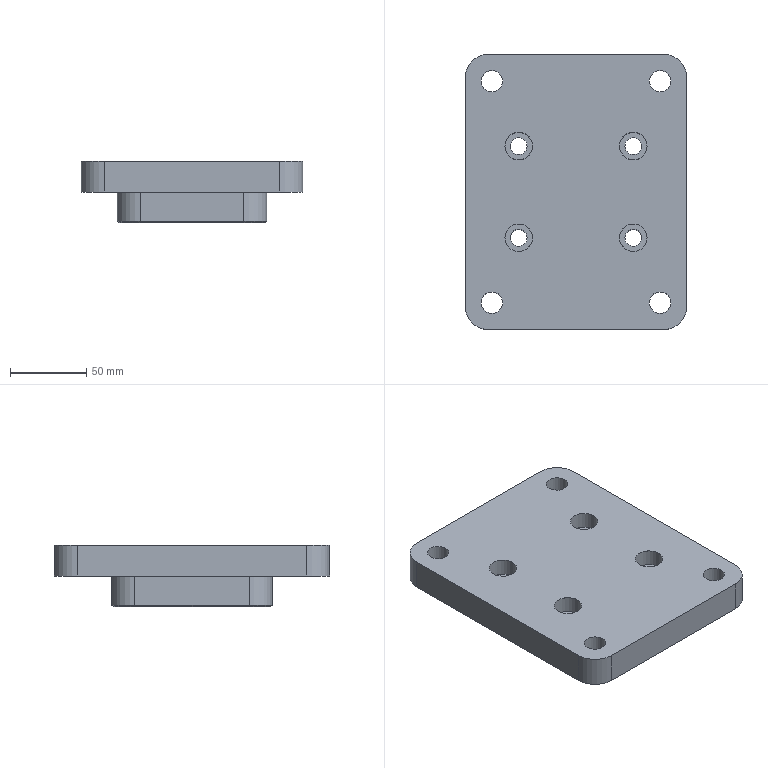NC program | NX | posted with a generic post | part box 145 x 180 x 40 mm
Lines 5548 to 5818 of 5818:
(HOLE_MILLING_COPY , TOOL : D10JING)
N11076 T11 M6
N11078 G54
N11080 G17 G0 G90 X-72.5 Y55. S5000 M3
N11082 G43 Z30. H11
N11084 Z0.5
N11086 G94 G3 X-73.5 Y54. R1. F1200.
N11088 X-72.5 Y53. R1.
N11090 X-72.5 Y53. Z-4.5 I0. J2.
N11092 X-72.5 Y53. Z-9.5 I0. J2.
N11094 X-72.5 Y53. Z-14.5 I0. J2.
N11096 X-72.5 Y53. Z-19.5 I0. J2.
N11098 X-71.324 Y53.382 Z-20. R2.
N11100 X-70.882 Y56.176 R2.
N11102 X-71.324 Y53.382 R-2.
N11104 X-71.103 Y54.779 R1.
N11106 X-72.5 Y55. R1.
N11108 G0 Z30.
N11110 X-30. Y37.5
N11112 Z0.5
N11114 G1 X-30.849 Y37.073
N11116 G3 X-30. Y33.5 R1.887
N11118 X-30. Y33.5 Z-4.5 I0. J4.
N11120 X-30. Y33.5 Z-9.5 I0. J4.
N11122 X-26.196 Y38.736 Z-11. R4.
N11124 X-31.236 Y41.304 R4.
N11126 X-26.196 Y38.736 R-4.
N11128 X-29.856 Y38.439 R1.887
N11130 G1 X-30. Y37.5
N11132 G0 Z30.
N11134 X30.
N11136 Z0.5
N11138 G1 X29.151 Y37.073
N11140 G3 X30. Y33.5 R1.887
N11142 X30. Y33.5 Z-4.5 I0. J4.
N11144 X30. Y33.5 Z-9.5 I0. J4.
N11146 X33.804 Y38.736 Z-11. R4.
N11148 X28.764 Y41.304 R4.
N11150 X33.804 Y38.736 R-4.
N11152 X30.144 Y38.439 R1.887
N11154 G1 X30. Y37.5
N11156 G0 Z30.
N11158 X72.5 Y55.
N11160 Z0.5
N11162 G3 X71.5 Y54. R1.
N11164 X72.5 Y53. R1.
N11166 X72.5 Y53. Z-4.5 I0. J2.
N11168 X72.5 Y53. Z-9.5 I0. J2.
N11170 X72.5 Y53. Z-14.5 I0. J2.
N11172 X72.5 Y53. Z-19.5 I0. J2.
N11174 X73.676 Y53.382 Z-20. R2.
N11176 X74.118 Y56.176 R2.
N11178 X73.676 Y53.382 R-2.
N11180 X73.897 Y54.779 R1.
N11182 X72.5 Y55. R1.
N11184 G0 Z30.
N11186 Y-55.
N11188 Z0.5
N11190 G3 X71.5 Y-56. R1.
N11192 X72.5 Y-57. R1.
N11194 X72.5 Y-57. Z-4.5 I0. J2.
N11196 X72.5 Y-57. Z-9.5 I0. J2.
N11198 X72.5 Y-57. Z-14.5 I0. J2.
N11200 X72.5 Y-57. Z-19.5 I0. J2.
N11202 X73.676 Y-56.618 Z-20. R2.
N11204 X74.118 Y-53.824 R2.
N11206 X73.676 Y-56.618 R-2.
N11208 X73.897 Y-55.221 R1.
N11210 X72.5 Y-55. R1.
N11212 G0 Z30.
N11214 X30. Y-37.5
N11216 Z0.5
N11218 G1 X29.151 Y-37.927
N11220 G3 X30. Y-41.5 R1.887
N11222 X30. Y-41.5 Z-4.5 I0. J4.
N11224 X30. Y-41.5 Z-9.5 I0. J4.
N11226 X33.804 Y-36.264 Z-11. R4.
N11228 X28.764 Y-33.696 R4.
N11230 X33.804 Y-36.264 R-4.
N11232 X30.144 Y-36.561 R1.887
N11234 G1 X30. Y-37.5
N11236 G0 Z30.
N11238 X-30.
N11240 Z0.5
N11242 G1 X-30.849 Y-37.927
N11244 G3 X-30. Y-41.5 R1.887
N11246 X-30. Y-41.5 Z-4.5 I0. J4.
N11248 X-30. Y-41.5 Z-9.5 I0. J4.
N11250 X-26.196 Y-36.264 Z-11. R4.
N11252 X-31.236 Y-33.696 R4.
N11254 X-26.196 Y-36.264 R-4.
N11256 X-29.856 Y-36.561 R1.887
N11258 G1 X-30. Y-37.5
N11260 G0 Z30.
N11262 X-72.5 Y-55.
N11264 Z0.5
N11266 G3 X-73.5 Y-56. R1.
N11268 X-72.5 Y-57. R1.
N11270 X-72.5 Y-57. Z-4.5 I0. J2.
N11272 X-72.5 Y-57. Z-9.5 I0. J2.
N11274 X-72.5 Y-57. Z-14.5 I0. J2.
N11276 X-72.5 Y-57. Z-19.5 I0. J2.
N11278 X-71.324 Y-56.618 Z-20. R2.
N11280 X-70.882 Y-53.824 R2.
N11282 X-71.324 Y-56.618 R-2.
N11284 X-71.103 Y-55.221 R1.
N11286 X-72.5 Y-55. R1.
N11288 G0 Z30.
(ZLEVEL_PROFILE_1 , TOOL : D10JING)
N11290 X97. Y-50.375
N11292 Z-18.
N11294 G1 Z-20. F1250.
N11296 X95.499 Y-51.242
N11298 G3 X95. Y-52.108 R1.
N11300 G1 Y-56.998
N11302 Y-57.5
N11304 G2 X75. Y-77.5 R20.
N11306 G1 X74.498
N11308 X69.608
N11310 G3 X68.742 Y-77.999 R1.
N11312 G1 X67.875 Y-79.5
N11314 Z-18.
N11316 G0 Z30.
N11318 Y79.5
N11320 Z-18.
N11322 G1 Z-20.
N11324 X68.742 Y77.999
N11326 G3 X69.608 Y77.499 R1.
N11328 G1 X74.053
N11330 X74.498 Y77.5
N11332 X75.
N11334 G2 X95. Y57.5 R20.
N11336 G1 Y56.998
N11338 Y52.108
N11340 G3 X95.499 Y51.242 R1.
N11342 G1 X97. Y50.375
N11344 Z-18.
N11346 G0 Z30.
N11348 X-97.
N11350 Z-18.
N11352 G1 Z-20.
N11354 X-95.499 Y51.242
N11356 G3 X-94.999 Y52.108 R1.
N11358 G1 Y56.553
N11360 X-95. Y56.998
N11362 Y57.5
N11364 G2 X-75. Y77.5 R20.
N11366 G1 X-74.498
N11368 X-74.053 Y77.499
N11370 X-69.608
N11372 G3 X-68.742 Y77.999 R1.
N11374 G1 X-67.875 Y79.5
N11376 Z-18.
N11378 G0 Z30.
N11380 Y-79.5
N11382 Z-18.
N11384 G1 Z-20.
N11386 X-68.742 Y-77.999
N11388 G3 X-69.608 Y-77.5 R1.
N11390 G1 X-74.498
N11392 X-75.
N11394 G2 X-95. Y-57.512 R20.
N11396 G1 Y-57.481
N11398 Y-56.998
N11400 X-94.999 Y-56.553
N11402 Y-52.108
N11404 G3 X-95.499 Y-51.242 R1.
N11406 G1 X-97. Y-50.375
N11408 Z-18.
N11410 G0 Z30.
N11412 M5
(PLANAR_MILL_COPY_COPY , TOOL : D6A45)
N11414 T07 M6
N11416 G54
N11418 G17 G0 G90 X73.266 Y60.343 S7500 M3
N11420 G43 Z30. H7
N11422 Z1.5
N11424 G94 G1 Z-1.5 F1250.
N11426 G3 X72.5 Y60.7 R1.
N11428 X66.8 Y55. R5.7
N11430 X72.5 Y60.7 R-5.7
N11432 X71.734 Y60.343 R1.
N11434 G1 Z1.5
N11436 G0 Z30.
N11438 X30.766 Y44.868
N11440 Z1.5
N11442 G1 Z-1.5
N11444 G3 X30. Y45.225 R1.
N11446 X22.275 Y37.5 R7.725
N11448 X30. Y45.225 R-7.725
N11450 X29.234 Y44.868 R1.
N11452 G1 Z1.5
N11454 G0 Z30.
N11456 X-29.234
N11458 Z1.5
N11460 G1 Z-1.5
N11462 G3 X-30. Y45.225 R1.
N11464 X-37.725 Y37.5 R7.725
N11466 X-30. Y45.225 R-7.725
N11468 X-30.766 Y44.868 R1.
N11470 G1 Z1.5
N11472 G0 Z30.
N11474 X-71.734 Y60.343
N11476 Z1.5
N11478 G1 Z-1.5
N11480 G3 X-72.5 Y60.7 R1.
N11482 X-78.2 Y55. R5.7
N11484 X-72.5 Y60.7 R-5.7
N11486 X-73.266 Y60.343 R1.
N11488 G1 Z1.5
N11490 G0 Z30.
N11492 X-77.843 Y-54.234
N11494 Z1.5
N11496 G1 Z-1.5
N11498 G3 X-78.2 Y-55. R1.
N11500 X-72.5 Y-60.7 R5.7
N11502 X-78.2 Y-55. R-5.7
N11504 X-77.843 Y-55.766 R1.
N11506 G1 Z1.5
N11508 G0 Z30.
N11510 X-30.766 Y-44.868
N11512 Z1.5
N11514 G1 Z-1.5
N11516 G3 X-30. Y-45.225 R1.
N11518 X-22.275 Y-37.5 R7.725
N11520 X-30. Y-45.225 R-7.725
N11522 X-29.234 Y-44.868 R1.
N11524 G1 Z1.5
N11526 G0 Z30.
N11528 X0.766 Y-74.157
N11530 Z1.5
N11532 G1 Z-1.5
N11534 G3 X0. Y-73.8 R1.
N11536 G1 X-75.
N11538 G2 X-91.3 Y-57.5 R16.3
N11540 G1 Y57.5
N11542 G2 X-75. Y73.8 R16.3
N11544 G1 X75.
N11546 G2 X91.3 Y57.5 R16.3
N11548 G1 Y-57.5
N11550 G2 X75. Y-73.8 R16.3
N11552 G1 X0.
N11554 G3 X-0.766 Y-74.157 R1.
N11556 G1 Z1.5
N11558 G0 Z30.
N11560 X29.234 Y-44.868
N11562 Z1.5
N11564 G1 Z-1.5
N11566 G3 X30. Y-45.225 R1.
N11568 X37.725 Y-37.5 R7.725
N11570 X30. Y-45.225 R-7.725
N11572 X30.766 Y-44.868 R1.
N11574 G1 Z1.5
N11576 G0 Z30.
N11578 X71.734 Y-60.343
N11580 Z1.5
N11582 G1 Z-1.5
N11584 G3 X72.5 Y-60.7 R1.
N11586 X78.2 Y-55. R5.7
N11588 X72.5 Y-60.7 R-5.7
N11590 X73.266 Y-60.343 R1.
N11592 G1 Z1.5
N11594 G0 Z30.
N11596 M5
N11598 M2